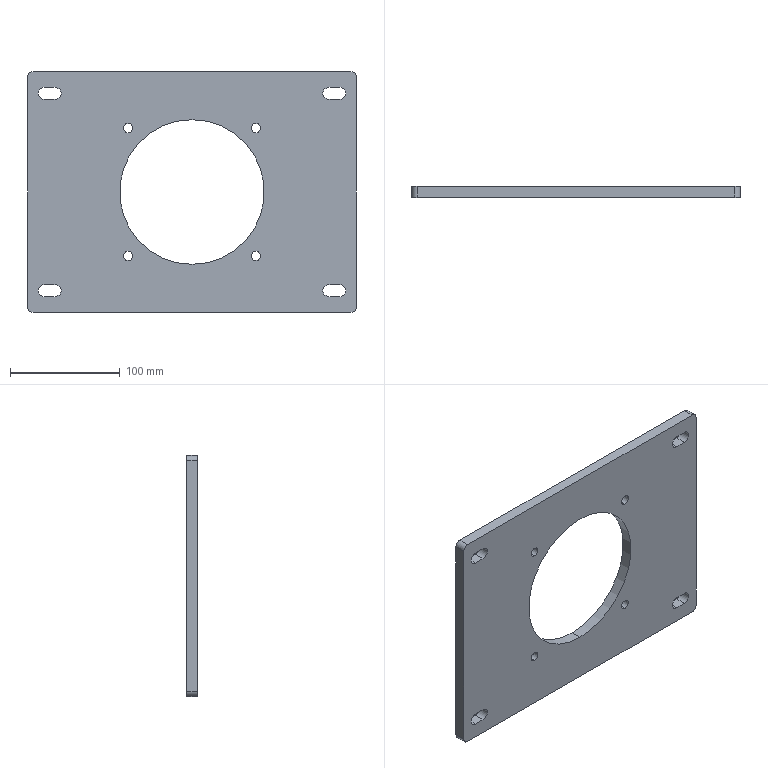Part | SolidWorks | features ICE 2, Extrusion 1, Fillet 1, HoleWzd 1 | 1 solid | 36 faces | box 300 x 10 x 220 mm | volume 512466 mm3 | cylinder 22 | plane 14 | commonest cylinder face diameters 8.5 x8 11 x8 10 x4 132 x2
STEP:
#1=CARTESIAN_POINT('',(-58.336,0.,-62.586));
#2=VERTEX_POINT('',#1);
#3=CARTESIAN_POINT('',(-58.336,0.,-54.086));
#4=VERTEX_POINT('',#3);
#5=CARTESIAN_POINT('',(-58.336,0.,-58.336));
#6=DIRECTION('',(0.,1.,0.));
#7=DIRECTION('',(0.,0.,1.));
#8=AXIS2_PLACEMENT_3D('',#5,#6,#7);
#9=CIRCLE('',#8,4.25);
#10=EDGE_CURVE('',#2,#4,#9,.T.);
#11=ORIENTED_EDGE('',*,*,#10,.F.);
#12=CARTESIAN_POINT('',(-58.336,10.,-62.586));
#13=VERTEX_POINT('',#12);
#14=CARTESIAN_POINT('',(-58.336,10.,-62.586));
#15=DIRECTION('',(0.,1.,0.));
#16=VECTOR('',#15,1000.);
#17=LINE('',#14,#16);
#18=EDGE_CURVE('',#2,#13,#17,.T.);
#19=ORIENTED_EDGE('',*,*,#18,.T.);
#20=CARTESIAN_POINT('',(-58.336,10.,-54.086));
#21=VERTEX_POINT('',#20);
#22=CARTESIAN_POINT('',(-58.336,10.,-58.336));
#23=DIRECTION('',(0.,1.,0.));
#24=DIRECTION('',(0.,0.,1.));
#25=AXIS2_PLACEMENT_3D('',#22,#23,#24);
#26=CIRCLE('',#25,4.25);
#27=EDGE_CURVE('',#13,#21,#26,.T.);
#28=ORIENTED_EDGE('',*,*,#27,.T.);
#29=CARTESIAN_POINT('',(-58.336,10.,-54.086));
#30=DIRECTION('',(0.,1.,0.));
#31=VECTOR('',#30,1000.);
#32=LINE('',#29,#31);
#33=EDGE_CURVE('',#4,#21,#32,.T.);
#34=ORIENTED_EDGE('',*,*,#33,.F.);
#35=EDGE_LOOP('',(#11,#19,#28,#34));
#36=FACE_OUTER_BOUND('',#35,.T.);
#37=CARTESIAN_POINT('',(-58.336,10.,-58.336));
#38=DIRECTION('',(0.,1.,0.));
#39=DIRECTION('',(0.,0.,1.));
#40=AXIS2_PLACEMENT_3D('',#37,#38,#39);
#41=CYLINDRICAL_SURFACE('',#40,4.25);
#42=ADVANCED_FACE('',(#36),#41,.F.);
#43=CARTESIAN_POINT('',(58.336,0.,-62.586));
#44=VERTEX_POINT('',#43);
#45=CARTESIAN_POINT('',(58.336,0.,-54.086));
#46=VERTEX_POINT('',#45);
#47=CARTESIAN_POINT('',(58.336,0.,-58.336));
#48=DIRECTION('',(0.,1.,0.));
#49=DIRECTION('',(0.,0.,1.));
#50=AXIS2_PLACEMENT_3D('',#47,#48,#49);
#51=CIRCLE('',#50,4.25);
#52=EDGE_CURVE('',#44,#46,#51,.T.);
#53=ORIENTED_EDGE('',*,*,#52,.F.);
#54=CARTESIAN_POINT('',(58.336,10.,-62.586));
#55=VERTEX_POINT('',#54);
#56=CARTESIAN_POINT('',(58.336,10.,-62.586));
#57=DIRECTION('',(0.,1.,0.));
#58=VECTOR('',#57,1000.);
#59=LINE('',#56,#58);
#60=EDGE_CURVE('',#44,#55,#59,.T.);
#61=ORIENTED_EDGE('',*,*,#60,.T.);
#62=CARTESIAN_POINT('',(58.336,10.,-54.086));
#63=VERTEX_POINT('',#62);
#64=CARTESIAN_POINT('',(58.336,10.,-58.336));
#65=DIRECTION('',(0.,1.,0.));
#66=DIRECTION('',(0.,0.,1.));
#67=AXIS2_PLACEMENT_3D('',#64,#65,#66);
#68=CIRCLE('',#67,4.25);
#69=EDGE_CURVE('',#55,#63,#68,.T.);
#70=ORIENTED_EDGE('',*,*,#69,.T.);
#71=CARTESIAN_POINT('',(58.336,10.,-54.086));
#72=DIRECTION('',(0.,1.,0.));
#73=VECTOR('',#72,1000.);
#74=LINE('',#71,#73);
#75=EDGE_CURVE('',#46,#63,#74,.T.);
#76=ORIENTED_EDGE('',*,*,#75,.F.);
#77=EDGE_LOOP('',(#53,#61,#70,#76));
#78=FACE_OUTER_BOUND('',#77,.T.);
#79=CARTESIAN_POINT('',(58.336,10.,-58.336));
#80=DIRECTION('',(0.,1.,0.));
#81=DIRECTION('',(0.,0.,1.));
#82=AXIS2_PLACEMENT_3D('',#79,#80,#81);
#83=CYLINDRICAL_SURFACE('',#82,4.25);
#84=ADVANCED_FACE('',(#78),#83,.F.);
#85=CARTESIAN_POINT('',(58.336,0.,54.086));
#86=VERTEX_POINT('',#85);
#87=CARTESIAN_POINT('',(58.336,0.,62.586));
#88=VERTEX_POINT('',#87);
#89=CARTESIAN_POINT('',(58.336,0.,58.336));
#90=DIRECTION('',(0.,1.,0.));
#91=DIRECTION('',(0.,0.,1.));
#92=AXIS2_PLACEMENT_3D('',#89,#90,#91);
#93=CIRCLE('',#92,4.25);
#94=EDGE_CURVE('',#86,#88,#93,.T.);
#95=ORIENTED_EDGE('',*,*,#94,.F.);
#96=CARTESIAN_POINT('',(58.336,10.,54.086));
#97=VERTEX_POINT('',#96);
#98=CARTESIAN_POINT('',(58.336,10.,54.086));
#99=DIRECTION('',(0.,1.,0.));
#100=VECTOR('',#99,1000.);
#101=LINE('',#98,#100);
#102=EDGE_CURVE('',#86,#97,#101,.T.);
#103=ORIENTED_EDGE('',*,*,#102,.T.);
#104=CARTESIAN_POINT('',(58.336,10.,62.586));
#105=VERTEX_POINT('',#104);
#106=CARTESIAN_POINT('',(58.336,10.,58.336));
#107=DIRECTION('',(0.,1.,0.));
#108=DIRECTION('',(0.,0.,1.));
#109=AXIS2_PLACEMENT_3D('',#106,#107,#108);
#110=CIRCLE('',#109,4.25);
#111=EDGE_CURVE('',#97,#105,#110,.T.);
#112=ORIENTED_EDGE('',*,*,#111,.T.);
#113=CARTESIAN_POINT('',(58.336,10.,62.586));
#114=DIRECTION('',(0.,1.,0.));
#115=VECTOR('',#114,1000.);
#116=LINE('',#113,#115);
#117=EDGE_CURVE('',#88,#105,#116,.T.);
#118=ORIENTED_EDGE('',*,*,#117,.F.);
#119=EDGE_LOOP('',(#95,#103,#112,#118));
#120=FACE_OUTER_BOUND('',#119,.T.);
#121=CARTESIAN_POINT('',(58.336,10.,58.336));
#122=DIRECTION('',(0.,1.,0.));
#123=DIRECTION('',(0.,0.,1.));
#124=AXIS2_PLACEMENT_3D('',#121,#122,#123);
#125=CYLINDRICAL_SURFACE('',#124,4.25);
#126=ADVANCED_FACE('',(#120),#125,.F.);
#127=CARTESIAN_POINT('',(-58.336,0.,54.086));
#128=VERTEX_POINT('',#127);
#129=CARTESIAN_POINT('',(-58.336,0.,62.586));
#130=VERTEX_POINT('',#129);
#131=CARTESIAN_POINT('',(-58.336,0.,58.336));
#132=DIRECTION('',(0.,1.,0.));
#133=DIRECTION('',(0.,0.,1.));
#134=AXIS2_PLACEMENT_3D('',#131,#132,#133);
#135=CIRCLE('',#134,4.25);
#136=EDGE_CURVE('',#128,#130,#135,.T.);
#137=ORIENTED_EDGE('',*,*,#136,.F.);
#138=CARTESIAN_POINT('',(-58.336,10.,54.086));
#139=VERTEX_POINT('',#138);
#140=CARTESIAN_POINT('',(-58.336,10.,54.086));
#141=DIRECTION('',(0.,1.,0.));
#142=VECTOR('',#141,1000.);
#143=LINE('',#140,#142);
#144=EDGE_CURVE('',#128,#139,#143,.T.);
#145=ORIENTED_EDGE('',*,*,#144,.T.);
#146=CARTESIAN_POINT('',(-58.336,10.,62.586));
#147=VERTEX_POINT('',#146);
#148=CARTESIAN_POINT('',(-58.336,10.,58.336));
#149=DIRECTION('',(0.,1.,0.));
#150=DIRECTION('',(0.,0.,1.));
#151=AXIS2_PLACEMENT_3D('',#148,#149,#150);
#152=CIRCLE('',#151,4.25);
#153=EDGE_CURVE('',#139,#147,#152,.T.);
#154=ORIENTED_EDGE('',*,*,#153,.T.);
#155=CARTESIAN_POINT('',(-58.336,10.,62.586));
#156=DIRECTION('',(0.,1.,0.));
#157=VECTOR('',#156,1000.);
#158=LINE('',#155,#157);
#159=EDGE_CURVE('',#130,#147,#158,.T.);
#160=ORIENTED_EDGE('',*,*,#159,.F.);
#161=EDGE_LOOP('',(#137,#145,#154,#160));
#162=FACE_OUTER_BOUND('',#161,.T.);
#163=CARTESIAN_POINT('',(-58.336,10.,58.336));
#164=DIRECTION('',(0.,1.,0.));
#165=DIRECTION('',(0.,0.,1.));
#166=AXIS2_PLACEMENT_3D('',#163,#164,#165);
#167=CYLINDRICAL_SURFACE('',#166,4.25);
#168=ADVANCED_FACE('',(#162),#167,.F.);
#169=CARTESIAN_POINT('',(0.,0.,-66.));
#170=VERTEX_POINT('',#169);
#171=CARTESIAN_POINT('',(0.,0.,66.));
#172=VERTEX_POINT('',#171);
#173=CARTESIAN_POINT('',(0.,0.,0.));
#174=DIRECTION('',(0.,1.,0.));
#175=DIRECTION('',(0.,0.,1.));
#176=AXIS2_PLACEMENT_3D('',#173,#174,#175);
#177=CIRCLE('',#176,66.);
#178=EDGE_CURVE('',#170,#172,#177,.T.);
#179=ORIENTED_EDGE('',*,*,#178,.F.);
#180=CARTESIAN_POINT('',(0.,10.,-66.));
#181=VERTEX_POINT('',#180);
#182=CARTESIAN_POINT('',(0.,0.,-66.));
#183=DIRECTION('',(0.,1.,0.));
#184=VECTOR('',#183,1000.);
#185=LINE('',#182,#184);
#186=EDGE_CURVE('',#170,#181,#185,.T.);
#187=ORIENTED_EDGE('',*,*,#186,.T.);
#188=CARTESIAN_POINT('',(0.,10.,66.));
#189=VERTEX_POINT('',#188);
#190=CARTESIAN_POINT('',(0.,10.,0.));
#191=DIRECTION('',(0.,1.,0.));
#192=DIRECTION('',(0.,0.,1.));
#193=AXIS2_PLACEMENT_3D('',#190,#191,#192);
#194=CIRCLE('',#193,66.);
#195=EDGE_CURVE('',#181,#189,#194,.T.);
#196=ORIENTED_EDGE('',*,*,#195,.T.);
#197=CARTESIAN_POINT('',(0.,0.,66.));
#198=DIRECTION('',(0.,1.,0.));
#199=VECTOR('',#198,1000.);
#200=LINE('',#197,#199);
#201=EDGE_CURVE('',#172,#189,#200,.T.);
#202=ORIENTED_EDGE('',*,*,#201,.F.);
#203=EDGE_LOOP('',(#179,#187,#196,#202));
#204=FACE_OUTER_BOUND('',#203,.T.);
#205=CARTESIAN_POINT('',(0.,0.,0.));
#206=DIRECTION('',(0.,1.,0.));
#207=DIRECTION('',(0.,0.,1.));
#208=AXIS2_PLACEMENT_3D('',#205,#206,#207);
#209=CYLINDRICAL_SURFACE('',#208,66.);
#210=ADVANCED_FACE('',(#204),#209,.F.);
#211=CARTESIAN_POINT('',(150.,10.,105.));
#212=VERTEX_POINT('',#211);
#213=CARTESIAN_POINT('',(150.,10.,-105.));
#214=VERTEX_POINT('',#213);
#215=CARTESIAN_POINT('',(150.,10.,-110.));
#216=DIRECTION('',(0.,0.,-1.));
#217=VECTOR('',#216,1000.);
#218=LINE('',#215,#217);
#219=EDGE_CURVE('',#212,#214,#218,.T.);
#220=ORIENTED_EDGE('',*,*,#219,.F.);
#221=CARTESIAN_POINT('',(150.,0.,105.));
#222=VERTEX_POINT('',#221);
#223=CARTESIAN_POINT('',(150.,10.,105.));
#224=DIRECTION('',(0.,-1.,0.));
#225=VECTOR('',#224,1000.);
#226=LINE('',#223,#225);
#227=EDGE_CURVE('',#212,#222,#226,.T.);
#228=ORIENTED_EDGE('',*,*,#227,.T.);
#229=CARTESIAN_POINT('',(150.,0.,-105.));
#230=VERTEX_POINT('',#229);
#231=CARTESIAN_POINT('',(150.,0.,-110.));
#232=DIRECTION('',(0.,0.,-1.));
#233=VECTOR('',#232,1000.);
#234=LINE('',#231,#233);
#235=EDGE_CURVE('',#222,#230,#234,.T.);
#236=ORIENTED_EDGE('',*,*,#235,.T.);
#237=CARTESIAN_POINT('',(150.,10.,-105.));
#238=DIRECTION('',(0.,1.,0.));
#239=VECTOR('',#238,1000.);
#240=LINE('',#237,#239);
#241=EDGE_CURVE('',#230,#214,#240,.T.);
#242=ORIENTED_EDGE('',*,*,#241,.T.);
#243=EDGE_LOOP('',(#220,#228,#236,#242));
#244=FACE_OUTER_BOUND('',#243,.T.);
#245=CARTESIAN_POINT('',(150.,10.,-110.));
#246=DIRECTION('',(-1.,0.,0.));
#247=DIRECTION('',(0.,0.,1.));
#248=AXIS2_PLACEMENT_3D('',#245,#246,#247);
#249=PLANE('',#248);
#250=ADVANCED_FACE('',(#244),#249,.F.);
#251=CARTESIAN_POINT('',(145.,10.,-110.));
#252=VERTEX_POINT('',#251);
#253=CARTESIAN_POINT('',(-145.,10.,-110.));
#254=VERTEX_POINT('',#253);
#255=CARTESIAN_POINT('',(-150.,10.,-110.));
#256=DIRECTION('',(-1.,0.,0.));
#257=VECTOR('',#256,1000.);
#258=LINE('',#255,#257);
#259=EDGE_CURVE('',#252,#254,#258,.T.);
#260=ORIENTED_EDGE('',*,*,#259,.F.);
#261=CARTESIAN_POINT('',(145.,0.,-110.));
#262=VERTEX_POINT('',#261);
#263=CARTESIAN_POINT('',(145.,10.,-110.));
#264=DIRECTION('',(0.,-1.,0.));
#265=VECTOR('',#264,1000.);
#266=LINE('',#263,#265);
#267=EDGE_CURVE('',#252,#262,#266,.T.);
#268=ORIENTED_EDGE('',*,*,#267,.T.);
#269=CARTESIAN_POINT('',(-145.,0.,-110.));
#270=VERTEX_POINT('',#269);
#271=CARTESIAN_POINT('',(-150.,0.,-110.));
#272=DIRECTION('',(-1.,0.,0.));
#273=VECTOR('',#272,1000.);
#274=LINE('',#271,#273);
#275=EDGE_CURVE('',#262,#270,#274,.T.);
#276=ORIENTED_EDGE('',*,*,#275,.T.);
#277=CARTESIAN_POINT('',(-145.,10.,-110.));
#278=DIRECTION('',(0.,1.,0.));
#279=VECTOR('',#278,1000.);
#280=LINE('',#277,#279);
#281=EDGE_CURVE('',#270,#254,#280,.T.);
#282=ORIENTED_EDGE('',*,*,#281,.T.);
#283=EDGE_LOOP('',(#260,#268,#276,#282));
#284=FACE_OUTER_BOUND('',#283,.T.);
#285=CARTESIAN_POINT('',(-150.,10.,-110.));
#286=DIRECTION('',(0.,0.,1.));
#287=DIRECTION('',(1.,0.,0.));
#288=AXIS2_PLACEMENT_3D('',#285,#286,#287);
#289=PLANE('',#288);
#290=ADVANCED_FACE('',(#284),#289,.F.);
#291=CARTESIAN_POINT('',(-150.,10.,-105.));
#292=VERTEX_POINT('',#291);
#293=CARTESIAN_POINT('',(-150.,10.,105.));
#294=VERTEX_POINT('',#293);
#295=CARTESIAN_POINT('',(-150.,10.,-110.));
#296=DIRECTION('',(0.,0.,1.));
#297=VECTOR('',#296,1000.);
#298=LINE('',#295,#297);
#299=EDGE_CURVE('',#292,#294,#298,.T.);
#300=ORIENTED_EDGE('',*,*,#299,.F.);
#301=CARTESIAN_POINT('',(-150.,0.,-105.));
#302=VERTEX_POINT('',#301);
#303=CARTESIAN_POINT('',(-150.,10.,-105.));
#304=DIRECTION('',(0.,-1.,0.));
#305=VECTOR('',#304,1000.);
#306=LINE('',#303,#305);
#307=EDGE_CURVE('',#292,#302,#306,.T.);
#308=ORIENTED_EDGE('',*,*,#307,.T.);
#309=CARTESIAN_POINT('',(-150.,0.,105.));
#310=VERTEX_POINT('',#309);
#311=CARTESIAN_POINT('',(-150.,0.,-110.));
#312=DIRECTION('',(0.,0.,1.));
#313=VECTOR('',#312,1000.);
#314=LINE('',#311,#313);
#315=EDGE_CURVE('',#302,#310,#314,.T.);
#316=ORIENTED_EDGE('',*,*,#315,.T.);
#317=CARTESIAN_POINT('',(-150.,10.,105.));
#318=DIRECTION('',(0.,1.,0.));
#319=VECTOR('',#318,1000.);
#320=LINE('',#317,#319);
#321=EDGE_CURVE('',#310,#294,#320,.T.);
#322=ORIENTED_EDGE('',*,*,#321,.T.);
#323=EDGE_LOOP('',(#300,#308,#316,#322));
#324=FACE_OUTER_BOUND('',#323,.T.);
#325=CARTESIAN_POINT('',(-150.,10.,-110.));
#326=DIRECTION('',(1.,0.,0.));
#327=DIRECTION('',(0.,0.,-1.));
#328=AXIS2_PLACEMENT_3D('',#325,#326,#327);
#329=PLANE('',#328);
#330=ADVANCED_FACE('',(#324),#329,.F.);
#331=CARTESIAN_POINT('',(-145.,0.,110.));
#332=VERTEX_POINT('',#331);
#333=CARTESIAN_POINT('',(145.,0.,110.));
#334=VERTEX_POINT('',#333);
#335=CARTESIAN_POINT('',(-150.,0.,110.));
#336=DIRECTION('',(1.,0.,0.));
#337=VECTOR('',#336,1000.);
#338=LINE('',#335,#337);
#339=EDGE_CURVE('',#332,#334,#338,.T.);
#340=ORIENTED_EDGE('',*,*,#339,.T.);
#341=CARTESIAN_POINT('',(145.,10.,110.));
#342=VERTEX_POINT('',#341);
#343=CARTESIAN_POINT('',(145.,10.,110.));
#344=DIRECTION('',(0.,1.,0.));
#345=VECTOR('',#344,1000.);
#346=LINE('',#343,#345);
#347=EDGE_CURVE('',#334,#342,#346,.T.);
#348=ORIENTED_EDGE('',*,*,#347,.T.);
#349=CARTESIAN_POINT('',(-145.,10.,110.));
#350=VERTEX_POINT('',#349);
#351=CARTESIAN_POINT('',(-150.,10.,110.));
#352=DIRECTION('',(1.,0.,0.));
#353=VECTOR('',#352,1000.);
#354=LINE('',#351,#353);
#355=EDGE_CURVE('',#350,#342,#354,.T.);
#356=ORIENTED_EDGE('',*,*,#355,.F.);
#357=CARTESIAN_POINT('',(-145.,10.,110.));
#358=DIRECTION('',(0.,-1.,0.));
#359=VECTOR('',#358,1000.);
#360=LINE('',#357,#359);
#361=EDGE_CURVE('',#350,#332,#360,.T.);
#362=ORIENTED_EDGE('',*,*,#361,.T.);
#363=EDGE_LOOP('',(#340,#348,#356,#362));
#364=FACE_OUTER_BOUND('',#363,.T.);
#365=CARTESIAN_POINT('',(-150.,10.,110.));
#366=DIRECTION('',(0.,0.,-1.));
#367=DIRECTION('',(-1.,0.,0.));
#368=AXIS2_PLACEMENT_3D('',#365,#366,#367);
#369=PLANE('',#368);
#370=ADVANCED_FACE('',(#364),#369,.F.);
#371=CARTESIAN_POINT('',(-135.,10.,84.5));
#372=VERTEX_POINT('',#371);
#373=CARTESIAN_POINT('',(-135.,10.,95.5));
#374=VERTEX_POINT('',#373);
#375=CARTESIAN_POINT('',(-135.,10.,90.));
#376=DIRECTION('',(0.,1.,0.));
#377=DIRECTION('',(0.,0.,-1.));
#378=AXIS2_PLACEMENT_3D('',#375,#376,#377);
#379=CIRCLE('',#378,5.5);
#380=EDGE_CURVE('',#372,#374,#379,.T.);
#381=ORIENTED_EDGE('',*,*,#380,.F.);
#382=CARTESIAN_POINT('',(-125.,10.,84.5));
#383=VERTEX_POINT('',#382);
#384=CARTESIAN_POINT('',(-135.,10.,84.5));
#385=DIRECTION('',(-1.,0.,0.));
#386=VECTOR('',#385,1000.);
#387=LINE('',#384,#386);
#388=EDGE_CURVE('',#383,#372,#387,.T.);
#389=ORIENTED_EDGE('',*,*,#388,.F.);
#390=CARTESIAN_POINT('',(-125.,10.,95.5));
#391=VERTEX_POINT('',#390);
#392=CARTESIAN_POINT('',(-125.,10.,90.));
#393=DIRECTION('',(0.,1.,0.));
#394=DIRECTION('',(0.,0.,-1.));
#395=AXIS2_PLACEMENT_3D('',#392,#393,#394);
#396=CIRCLE('',#395,5.5);
#397=EDGE_CURVE('',#391,#383,#396,.T.);
#398=ORIENTED_EDGE('',*,*,#397,.F.);
#399=CARTESIAN_POINT('',(-135.,10.,95.5));
#400=DIRECTION('',(1.,0.,0.));
#401=VECTOR('',#400,1000.);
#402=LINE('',#399,#401);
#403=EDGE_CURVE('',#374,#391,#402,.T.);
#404=ORIENTED_EDGE('',*,*,#403,.F.);
#405=EDGE_LOOP('',(#381,#389,#398,#404));
#406=FACE_BOUND('',#405,.T.);
#407=CARTESIAN_POINT('',(135.,10.,95.5));
#408=VERTEX_POINT('',#407);
#409=CARTESIAN_POINT('',(135.,10.,84.5));
#410=VERTEX_POINT('',#409);
#411=CARTESIAN_POINT('',(135.,10.,90.));
#412=DIRECTION('',(0.,1.,0.));
#413=DIRECTION('',(0.,0.,1.));
#414=AXIS2_PLACEMENT_3D('',#411,#412,#413);
#415=CIRCLE('',#414,5.5);
#416=EDGE_CURVE('',#408,#410,#415,.T.);
#417=ORIENTED_EDGE('',*,*,#416,.F.);
#418=CARTESIAN_POINT('',(125.,10.,95.5));
#419=VERTEX_POINT('',#418);
#420=CARTESIAN_POINT('',(135.,10.,95.5));
#421=DIRECTION('',(1.,0.,0.));
#422=VECTOR('',#421,1000.);
#423=LINE('',#420,#422);
#424=EDGE_CURVE('',#419,#408,#423,.T.);
#425=ORIENTED_EDGE('',*,*,#424,.F.);
#426=CARTESIAN_POINT('',(125.,10.,84.5));
#427=VERTEX_POINT('',#426);
#428=CARTESIAN_POINT('',(125.,10.,90.));
#429=DIRECTION('',(0.,1.,0.));
#430=DIRECTION('',(0.,0.,1.));
#431=AXIS2_PLACEMENT_3D('',#428,#429,#430);
#432=CIRCLE('',#431,5.5);
#433=EDGE_CURVE('',#427,#419,#432,.T.);
#434=ORIENTED_EDGE('',*,*,#433,.F.);
#435=CARTESIAN_POINT('',(135.,10.,84.5));
#436=DIRECTION('',(-1.,0.,0.));
#437=VECTOR('',#436,1000.);
#438=LINE('',#435,#437);
#439=EDGE_CURVE('',#410,#427,#438,.T.);
#440=ORIENTED_EDGE('',*,*,#439,.F.);
#441=EDGE_LOOP('',(#417,#425,#434,#440));
#442=FACE_BOUND('',#441,.T.);
#443=CARTESIAN_POINT('',(135.,10.,-84.5));
#444=VERTEX_POINT('',#443);
#445=CARTESIAN_POINT('',(135.,10.,-95.5));
#446=VERTEX_POINT('',#445);
#447=CARTESIAN_POINT('',(135.,10.,-90.));
#448=DIRECTION('',(0.,1.,0.));
#449=DIRECTION('',(0.,0.,-1.));
#450=AXIS2_PLACEMENT_3D('',#447,#448,#449);
#451=CIRCLE('',#450,5.5);
#452=EDGE_CURVE('',#444,#446,#451,.T.);
#453=ORIENTED_EDGE('',*,*,#452,.F.);
#454=CARTESIAN_POINT('',(125.,10.,-84.5));
#455=VERTEX_POINT('',#454);
#456=CARTESIAN_POINT('',(135.,10.,-84.5));
#457=DIRECTION('',(1.,0.,0.));
#458=VECTOR('',#457,1000.);
#459=LINE('',#456,#458);
#460=EDGE_CURVE('',#455,#444,#459,.T.);
#461=ORIENTED_EDGE('',*,*,#460,.F.);
#462=CARTESIAN_POINT('',(125.,10.,-95.5));
#463=VERTEX_POINT('',#462);
#464=CARTESIAN_POINT('',(125.,10.,-90.));
#465=DIRECTION('',(0.,1.,0.));
#466=DIRECTION('',(0.,0.,-1.));
#467=AXIS2_PLACEMENT_3D('',#464,#465,#466);
#468=CIRCLE('',#467,5.5);
#469=EDGE_CURVE('',#463,#455,#468,.T.);
#470=ORIENTED_EDGE('',*,*,#469,.F.);
#471=CARTESIAN_POINT('',(135.,10.,-95.5));
#472=DIRECTION('',(-1.,0.,0.));
#473=VECTOR('',#472,1000.);
#474=LINE('',#471,#473);
#475=EDGE_CURVE('',#446,#463,#474,.T.);
#476=ORIENTED_EDGE('',*,*,#475,.F.);
#477=EDGE_LOOP('',(#453,#461,#470,#476));
#478=FACE_BOUND('',#477,.T.);
#479=CARTESIAN_POINT('',(-135.,10.,-95.5));
#480=VERTEX_POINT('',#479);
#481=CARTESIAN_POINT('',(-135.,10.,-84.5));
#482=VERTEX_POINT('',#481);
#483=CARTESIAN_POINT('',(-135.,10.,-90.));
#484=DIRECTION('',(0.,1.,0.));
#485=DIRECTION('',(0.,0.,1.));
#486=AXIS2_PLACEMENT_3D('',#483,#484,#485);
#487=CIRCLE('',#486,5.5);
#488=EDGE_CURVE('',#480,#482,#487,.T.);
#489=ORIENTED_EDGE('',*,*,#488,.F.);
#490=CARTESIAN_POINT('',(-125.,10.,-95.5));
#491=VERTEX_POINT('',#490);
#492=CARTESIAN_POINT('',(-135.,10.,-95.5));
#493=DIRECTION('',(-1.,0.,0.));
#494=VECTOR('',#493,1000.);
#495=LINE('',#492,#494);
#496=EDGE_CURVE('',#491,#480,#495,.T.);
#497=ORIENTED_EDGE('',*,*,#496,.F.);
#498=CARTESIAN_POINT('',(-125.,10.,-84.5));
#499=VERTEX_POINT('',#498);
#500=CARTESIAN_POINT('',(-125.,10.,-90.));
#501=DIRECTION('',(0.,1.,0.));
#502=DIRECTION('',(0.,0.,1.));
#503=AXIS2_PLACEMENT_3D('',#500,#501,#502);
#504=CIRCLE('',#503,5.5);
#505=EDGE_CURVE('',#499,#491,#504,.T.);
#506=ORIENTED_EDGE('',*,*,#505,.F.);
#507=CARTESIAN_POINT('',(-135.,10.,-84.5));
#508=DIRECTION('',(1.,0.,0.));
#509=VECTOR('',#508,1000.);
#510=LINE('',#507,#509);
#511=EDGE_CURVE('',#482,#499,#510,.T.);
#512=ORIENTED_EDGE('',*,*,#511,.F.);
#513=EDGE_LOOP('',(#489,#497,#506,#512));
#514=FACE_BOUND('',#513,.T.);
#515=CARTESIAN_POINT('',(-58.336,10.,-58.336));
#516=DIRECTION('',(0.,1.,0.));
#517=DIRECTION('',(0.,0.,1.));
#518=AXIS2_PLACEMENT_3D('',#515,#516,#517);
#519=CIRCLE('',#518,4.25);
#520=EDGE_CURVE('',#21,#13,#519,.T.);
#521=ORIENTED_EDGE('',*,*,#520,.F.);
#522=ORIENTED_EDGE('',*,*,#27,.F.);
#523=EDGE_LOOP('',(#521,#522));
#524=FACE_BOUND('',#523,.T.);
#525=CARTESIAN_POINT('',(58.336,10.,-58.336));
#526=DIRECTION('',(0.,1.,0.));
#527=DIRECTION('',(0.,0.,1.));
#528=AXIS2_PLACEMENT_3D('',#525,#526,#527);
#529=CIRCLE('',#528,4.25);
#530=EDGE_CURVE('',#63,#55,#529,.T.);
#531=ORIENTED_EDGE('',*,*,#530,.F.);
#532=ORIENTED_EDGE('',*,*,#69,.F.);
#533=EDGE_LOOP('',(#531,#532));
#534=FACE_BOUND('',#533,.T.);
#535=CARTESIAN_POINT('',(58.336,10.,58.336));
#536=DIRECTION('',(0.,1.,0.));
#537=DIRECTION('',(0.,0.,1.));
#538=AXIS2_PLACEMENT_3D('',#535,#536,#537);
#539=CIRCLE('',#538,4.25);
#540=EDGE_CURVE('',#105,#97,#539,.T.);
#541=ORIENTED_EDGE('',*,*,#540,.F.);
#542=ORIENTED_EDGE('',*,*,#111,.F.);
#543=EDGE_LOOP('',(#541,#542));
#544=FACE_BOUND('',#543,.T.);
#545=CARTESIAN_POINT('',(-58.336,10.,58.336));
#546=DIRECTION('',(0.,1.,0.));
#547=DIRECTION('',(0.,0.,1.));
#548=AXIS2_PLACEMENT_3D('',#545,#546,#547);
#549=CIRCLE('',#548,4.25);
#550=EDGE_CURVE('',#147,#139,#549,.T.);
#551=ORIENTED_EDGE('',*,*,#550,.F.);
#552=ORIENTED_EDGE('',*,*,#153,.F.);
#553=EDGE_LOOP('',(#551,#552));
#554=FACE_BOUND('',#553,.T.);
#555=CARTESIAN_POINT('',(0.,10.,0.));
#556=DIRECTION('',(0.,1.,0.));
#557=DIRECTION('',(0.,0.,1.));
#558=AXIS2_PLACEMENT_3D('',#555,#556,#557);
#559=CIRCLE('',#558,66.);
#560=EDGE_CURVE('',#189,#181,#559,.T.);
#561=ORIENTED_EDGE('',*,*,#560,.F.);
#562=ORIENTED_EDGE('',*,*,#195,.F.);
#563=EDGE_LOOP('',(#561,#562));
#564=FACE_BOUND('',#563,.T.);
#565=ORIENTED_EDGE('',*,*,#355,.T.);
#566=CARTESIAN_POINT('',(145.,10.,105.));
#567=DIRECTION('',(0.,1.,0.));
#568=DIRECTION('',(0.,0.,1.));
#569=AXIS2_PLACEMENT_3D('',#566,#567,#568);
#570=CIRCLE('',#569,5.);
#571=EDGE_CURVE('',#342,#212,#570,.T.);
#572=ORIENTED_EDGE('',*,*,#571,.T.);
#573=ORIENTED_EDGE('',*,*,#219,.T.);
#574=CARTESIAN_POINT('',(145.,10.,-105.));
#575=DIRECTION('',(0.,1.,0.));
#576=DIRECTION('',(0.,0.,1.));
#577=AXIS2_PLACEMENT_3D('',#574,#575,#576);
#578=CIRCLE('',#577,5.);
#579=EDGE_CURVE('',#214,#252,#578,.T.);
#580=ORIENTED_EDGE('',*,*,#579,.T.);
#581=ORIENTED_EDGE('',*,*,#259,.T.);
#582=CARTESIAN_POINT('',(-145.,10.,-105.));
#583=DIRECTION('',(0.,1.,0.));
#584=DIRECTION('',(0.,0.,1.));
#585=AXIS2_PLACEMENT_3D('',#582,#583,#584);
#586=CIRCLE('',#585,5.);
#587=EDGE_CURVE('',#254,#292,#586,.T.);
#588=ORIENTED_EDGE('',*,*,#587,.T.);
#589=ORIENTED_EDGE('',*,*,#299,.T.);
#590=CARTESIAN_POINT('',(-145.,10.,105.));
#591=DIRECTION('',(0.,1.,0.));
#592=DIRECTION('',(0.,0.,1.));
#593=AXIS2_PLACEMENT_3D('',#590,#591,#592);
#594=CIRCLE('',#593,5.);
#595=EDGE_CURVE('',#294,#350,#594,.T.);
#596=ORIENTED_EDGE('',*,*,#595,.T.);
#597=EDGE_LOOP('',(#565,#572,#573,#580,#581,#588,#589,#596));
#598=FACE_OUTER_BOUND('',#597,.T.);
#599=CARTESIAN_POINT('',(0.,10.,0.));
#600=DIRECTION('',(0.,1.,0.));
#601=DIRECTION('',(0.,0.,1.));
#602=AXIS2_PLACEMENT_3D('',#599,#600,#601);
#603=PLANE('',#602);
#604=ADVANCED_FACE('',(#406,#442,#478,#514,#524,#534,#544,#554,#564,#598),#603,.T.);
#605=CARTESIAN_POINT('',(-125.,0.,84.5));
#606=VERTEX_POINT('',#605);
#607=CARTESIAN_POINT('',(-135.,0.,84.5));
#608=VERTEX_POINT('',#607);
#609=CARTESIAN_POINT('',(-135.,0.,84.5));
#610=DIRECTION('',(-1.,0.,0.));
#611=VECTOR('',#610,1000.);
#612=LINE('',#609,#611);
#613=EDGE_CURVE('',#606,#608,#612,.T.);
#614=ORIENTED_EDGE('',*,*,#613,.T.);
#615=CARTESIAN_POINT('',(-135.,0.,95.5));
#616=VERTEX_POINT('',#615);
#617=CARTESIAN_POINT('',(-135.,0.,90.));
#618=DIRECTION('',(0.,1.,0.));
#619=DIRECTION('',(0.,0.,-1.));
#620=AXIS2_PLACEMENT_3D('',#617,#618,#619);
#621=CIRCLE('',#620,5.5);
#622=EDGE_CURVE('',#608,#616,#621,.T.);
#623=ORIENTED_EDGE('',*,*,#622,.T.);
#624=CARTESIAN_POINT('',(-125.,0.,95.5));
#625=VERTEX_POINT('',#624);
#626=CARTESIAN_POINT('',(-135.,0.,95.5));
#627=DIRECTION('',(1.,0.,0.));
#628=VECTOR('',#627,1000.);
#629=LINE('',#626,#628);
#630=EDGE_CURVE('',#616,#625,#629,.T.);
#631=ORIENTED_EDGE('',*,*,#630,.T.);
#632=CARTESIAN_POINT('',(-125.,0.,90.));
#633=DIRECTION('',(0.,1.,0.));
#634=DIRECTION('',(0.,0.,-1.));
#635=AXIS2_PLACEMENT_3D('',#632,#633,#634);
#636=CIRCLE('',#635,5.5);
#637=EDGE_CURVE('',#625,#606,#636,.T.);
#638=ORIENTED_EDGE('',*,*,#637,.T.);
#639=EDGE_LOOP('',(#614,#623,#631,#638));
#640=FACE_BOUND('',#639,.T.);
#641=CARTESIAN_POINT('',(125.,0.,95.5));
#642=VERTEX_POINT('',#641);
#643=CARTESIAN_POINT('',(135.,0.,95.5));
#644=VERTEX_POINT('',#643);
#645=CARTESIAN_POINT('',(135.,0.,95.5));
#646=DIRECTION('',(1.,0.,0.));
#647=VECTOR('',#646,1000.);
#648=LINE('',#645,#647);
#649=EDGE_CURVE('',#642,#644,#648,.T.);
#650=ORIENTED_EDGE('',*,*,#649,.T.);
#651=CARTESIAN_POINT('',(135.,0.,84.5));
#652=VERTEX_POINT('',#651);
#653=CARTESIAN_POINT('',(135.,0.,90.));
#654=DIRECTION('',(0.,1.,0.));
#655=DIRECTION('',(0.,0.,1.));
#656=AXIS2_PLACEMENT_3D('',#653,#654,#655);
#657=CIRCLE('',#656,5.5);
#658=EDGE_CURVE('',#644,#652,#657,.T.);
#659=ORIENTED_EDGE('',*,*,#658,.T.);
#660=CARTESIAN_POINT('',(125.,0.,84.5));
#661=VERTEX_POINT('',#660);
#662=CARTESIAN_POINT('',(135.,0.,84.5));
#663=DIRECTION('',(-1.,0.,0.));
#664=VECTOR('',#663,1000.);
#665=LINE('',#662,#664);
#666=EDGE_CURVE('',#652,#661,#665,.T.);
#667=ORIENTED_EDGE('',*,*,#666,.T.);
#668=CARTESIAN_POINT('',(125.,0.,90.));
#669=DIRECTION('',(0.,1.,0.));
#670=DIRECTION('',(0.,0.,1.));
#671=AXIS2_PLACEMENT_3D('',#668,#669,#670);
#672=CIRCLE('',#671,5.5);
#673=EDGE_CURVE('',#661,#642,#672,.T.);
#674=ORIENTED_EDGE('',*,*,#673,.T.);
#675=EDGE_LOOP('',(#650,#659,#667,#674));
#676=FACE_BOUND('',#675,.T.);
#677=CARTESIAN_POINT('',(125.,0.,-84.5));
#678=VERTEX_POINT('',#677);
#679=CARTESIAN_POINT('',(135.,0.,-84.5));
#680=VERTEX_POINT('',#679);
#681=CARTESIAN_POINT('',(135.,0.,-84.5));
#682=DIRECTION('',(1.,0.,0.));
#683=VECTOR('',#682,1000.);
#684=LINE('',#681,#683);
#685=EDGE_CURVE('',#678,#680,#684,.T.);
#686=ORIENTED_EDGE('',*,*,#685,.T.);
#687=CARTESIAN_POINT('',(135.,0.,-95.5));
#688=VERTEX_POINT('',#687);
#689=CARTESIAN_POINT('',(135.,0.,-90.));
#690=DIRECTION('',(0.,1.,0.));
#691=DIRECTION('',(0.,0.,-1.));
#692=AXIS2_PLACEMENT_3D('',#689,#690,#691);
#693=CIRCLE('',#692,5.5);
#694=EDGE_CURVE('',#680,#688,#693,.T.);
#695=ORIENTED_EDGE('',*,*,#694,.T.);
#696=CARTESIAN_POINT('',(125.,0.,-95.5));
#697=VERTEX_POINT('',#696);
#698=CARTESIAN_POINT('',(135.,0.,-95.5));
#699=DIRECTION('',(-1.,0.,0.));
#700=VECTOR('',#699,1000.);
#701=LINE('',#698,#700);
#702=EDGE_CURVE('',#688,#697,#701,.T.);
#703=ORIENTED_EDGE('',*,*,#702,.T.);
#704=CARTESIAN_POINT('',(125.,0.,-90.));
#705=DIRECTION('',(0.,1.,0.));
#706=DIRECTION('',(0.,0.,-1.));
#707=AXIS2_PLACEMENT_3D('',#704,#705,#706);
#708=CIRCLE('',#707,5.5);
#709=EDGE_CURVE('',#697,#678,#708,.T.);
#710=ORIENTED_EDGE('',*,*,#709,.T.);
#711=EDGE_LOOP('',(#686,#695,#703,#710));
#712=FACE_BOUND('',#711,.T.);
#713=CARTESIAN_POINT('',(-125.,0.,-95.5));
#714=VERTEX_POINT('',#713);
#715=CARTESIAN_POINT('',(-135.,0.,-95.5));
#716=VERTEX_POINT('',#715);
#717=CARTESIAN_POINT('',(-135.,0.,-95.5));
#718=DIRECTION('',(-1.,0.,0.));
#719=VECTOR('',#718,1000.);
#720=LINE('',#717,#719);
#721=EDGE_CURVE('',#714,#716,#720,.T.);
#722=ORIENTED_EDGE('',*,*,#721,.T.);
#723=CARTESIAN_POINT('',(-135.,0.,-84.5));
#724=VERTEX_POINT('',#723);
#725=CARTESIAN_POINT('',(-135.,0.,-90.));
#726=DIRECTION('',(0.,1.,0.));
#727=DIRECTION('',(0.,0.,1.));
#728=AXIS2_PLACEMENT_3D('',#725,#726,#727);
#729=CIRCLE('',#728,5.5);
#730=EDGE_CURVE('',#716,#724,#729,.T.);
#731=ORIENTED_EDGE('',*,*,#730,.T.);
#732=CARTESIAN_POINT('',(-125.,0.,-84.5));
#733=VERTEX_POINT('',#732);
#734=CARTESIAN_POINT('',(-135.,0.,-84.5));
#735=DIRECTION('',(1.,0.,0.));
#736=VECTOR('',#735,1000.);
#737=LINE('',#734,#736);
#738=EDGE_CURVE('',#724,#733,#737,.T.);
#739=ORIENTED_EDGE('',*,*,#738,.T.);
#740=CARTESIAN_POINT('',(-125.,0.,-90.));
#741=DIRECTION('',(0.,1.,0.));
#742=DIRECTION('',(0.,0.,1.));
#743=AXIS2_PLACEMENT_3D('',#740,#741,#742);
#744=CIRCLE('',#743,5.5);
#745=EDGE_CURVE('',#733,#714,#744,.T.);
#746=ORIENTED_EDGE('',*,*,#745,.T.);
#747=EDGE_LOOP('',(#722,#731,#739,#746));
#748=FACE_BOUND('',#747,.T.);
#749=CARTESIAN_POINT('',(-58.336,0.,-58.336));
#750=DIRECTION('',(0.,1.,0.));
#751=DIRECTION('',(0.,0.,1.));
#752=AXIS2_PLACEMENT_3D('',#749,#750,#751);
#753=CIRCLE('',#752,4.25);
#754=EDGE_CURVE('',#4,#2,#753,.T.);
#755=ORIENTED_EDGE('',*,*,#754,.T.);
#756=ORIENTED_EDGE('',*,*,#10,.T.);
#757=EDGE_LOOP('',(#755,#756));
#758=FACE_BOUND('',#757,.T.);
#759=CARTESIAN_POINT('',(58.336,0.,-58.336));
#760=DIRECTION('',(0.,1.,0.));
#761=DIRECTION('',(0.,0.,1.));
#762=AXIS2_PLACEMENT_3D('',#759,#760,#761);
#763=CIRCLE('',#762,4.25);
#764=EDGE_CURVE('',#46,#44,#763,.T.);
#765=ORIENTED_EDGE('',*,*,#764,.T.);
#766=ORIENTED_EDGE('',*,*,#52,.T.);
#767=EDGE_LOOP('',(#765,#766));
#768=FACE_BOUND('',#767,.T.);
#769=CARTESIAN_POINT('',(58.336,0.,58.336));
#770=DIRECTION('',(0.,1.,0.));
#771=DIRECTION('',(0.,0.,1.));
#772=AXIS2_PLACEMENT_3D('',#769,#770,#771);
#773=CIRCLE('',#772,4.25);
#774=EDGE_CURVE('',#88,#86,#773,.T.);
#775=ORIENTED_EDGE('',*,*,#774,.T.);
#776=ORIENTED_EDGE('',*,*,#94,.T.);
#777=EDGE_LOOP('',(#775,#776));
#778=FACE_BOUND('',#777,.T.);
#779=CARTESIAN_POINT('',(-58.336,0.,58.336));
#780=DIRECTION('',(0.,1.,0.));
#781=DIRECTION('',(0.,0.,1.));
#782=AXIS2_PLACEMENT_3D('',#779,#780,#781);
#783=CIRCLE('',#782,4.25);
#784=EDGE_CURVE('',#130,#128,#783,.T.);
#785=ORIENTED_EDGE('',*,*,#784,.T.);
#786=ORIENTED_EDGE('',*,*,#136,.T.);
#787=EDGE_LOOP('',(#785,#786));
#788=FACE_BOUND('',#787,.T.);
#789=CARTESIAN_POINT('',(0.,0.,0.));
#790=DIRECTION('',(0.,1.,0.));
#791=DIRECTION('',(0.,0.,1.));
#792=AXIS2_PLACEMENT_3D('',#789,#790,#791);
#793=CIRCLE('',#792,66.);
#794=EDGE_CURVE('',#172,#170,#793,.T.);
#795=ORIENTED_EDGE('',*,*,#794,.T.);
#796=ORIENTED_EDGE('',*,*,#178,.T.);
#797=EDGE_LOOP('',(#795,#796));
#798=FACE_BOUND('',#797,.T.);
#799=ORIENTED_EDGE('',*,*,#235,.F.);
#800=CARTESIAN_POINT('',(145.,0.,105.));
#801=DIRECTION('',(0.,-1.,0.));
#802=DIRECTION('',(0.,0.,1.));
#803=AXIS2_PLACEMENT_3D('',#800,#801,#802);
#804=CIRCLE('',#803,5.);
#805=EDGE_CURVE('',#222,#334,#804,.T.);
#806=ORIENTED_EDGE('',*,*,#805,.T.);
#807=ORIENTED_EDGE('',*,*,#339,.F.);
#808=CARTESIAN_POINT('',(-145.,0.,105.));
#809=DIRECTION('',(0.,-1.,0.));
#810=DIRECTION('',(0.,0.,1.));
#811=AXIS2_PLACEMENT_3D('',#808,#809,#810);
#812=CIRCLE('',#811,5.);
#813=EDGE_CURVE('',#332,#310,#812,.T.);
#814=ORIENTED_EDGE('',*,*,#813,.T.);
#815=ORIENTED_EDGE('',*,*,#315,.F.);
#816=CARTESIAN_POINT('',(-145.,0.,-105.));
#817=DIRECTION('',(0.,-1.,0.));
#818=DIRECTION('',(0.,0.,1.));
#819=AXIS2_PLACEMENT_3D('',#816,#817,#818);
#820=CIRCLE('',#819,5.);
#821=EDGE_CURVE('',#302,#270,#820,.T.);
#822=ORIENTED_EDGE('',*,*,#821,.T.);
#823=ORIENTED_EDGE('',*,*,#275,.F.);
#824=CARTESIAN_POINT('',(145.,0.,-105.));
#825=DIRECTION('',(0.,-1.,0.));
#826=DIRECTION('',(0.,0.,1.));
#827=AXIS2_PLACEMENT_3D('',#824,#825,#826);
#828=CIRCLE('',#827,5.);
#829=EDGE_CURVE('',#262,#230,#828,.T.);
#830=ORIENTED_EDGE('',*,*,#829,.T.);
#831=EDGE_LOOP('',(#799,#806,#807,#814,#815,#822,#823,#830));
#832=FACE_OUTER_BOUND('',#831,.T.);
#833=CARTESIAN_POINT('',(0.,0.,0.));
#834=DIRECTION('',(0.,1.,0.));
#835=DIRECTION('',(0.,0.,1.));
#836=AXIS2_PLACEMENT_3D('',#833,#834,#835);
#837=PLANE('',#836);
#838=ADVANCED_FACE('',(#640,#676,#712,#748,#758,#768,#778,#788,#798,#832),#837,.F.);
#839=ORIENTED_EDGE('',*,*,#186,.F.);
#840=ORIENTED_EDGE('',*,*,#794,.F.);
#841=ORIENTED_EDGE('',*,*,#201,.T.);
#842=ORIENTED_EDGE('',*,*,#560,.T.);
#843=EDGE_LOOP('',(#839,#840,#841,#842));
#844=FACE_OUTER_BOUND('',#843,.T.);
#845=CARTESIAN_POINT('',(0.,0.,0.));
#846=DIRECTION('',(0.,1.,0.));
#847=DIRECTION('',(0.,0.,1.));
#848=AXIS2_PLACEMENT_3D('',#845,#846,#847);
#849=CYLINDRICAL_SURFACE('',#848,66.);
#850=ADVANCED_FACE('',(#844),#849,.F.);
#851=ORIENTED_EDGE('',*,*,#144,.F.);
#852=ORIENTED_EDGE('',*,*,#784,.F.);
#853=ORIENTED_EDGE('',*,*,#159,.T.);
#854=ORIENTED_EDGE('',*,*,#550,.T.);
#855=EDGE_LOOP('',(#851,#852,#853,#854));
#856=FACE_OUTER_BOUND('',#855,.T.);
#857=CARTESIAN_POINT('',(-58.336,10.,58.336));
#858=DIRECTION('',(0.,1.,0.));
#859=DIRECTION('',(0.,0.,1.));
#860=AXIS2_PLACEMENT_3D('',#857,#858,#859);
#861=CYLINDRICAL_SURFACE('',#860,4.25);
#862=ADVANCED_FACE('',(#856),#861,.F.);
#863=ORIENTED_EDGE('',*,*,#102,.F.);
#864=ORIENTED_EDGE('',*,*,#774,.F.);
#865=ORIENTED_EDGE('',*,*,#117,.T.);
#866=ORIENTED_EDGE('',*,*,#540,.T.);
#867=EDGE_LOOP('',(#863,#864,#865,#866));
#868=FACE_OUTER_BOUND('',#867,.T.);
#869=CARTESIAN_POINT('',(58.336,10.,58.336));
#870=DIRECTION('',(0.,1.,0.));
#871=DIRECTION('',(0.,0.,1.));
#872=AXIS2_PLACEMENT_3D('',#869,#870,#871);
#873=CYLINDRICAL_SURFACE('',#872,4.25);
#874=ADVANCED_FACE('',(#868),#873,.F.);
#875=ORIENTED_EDGE('',*,*,#60,.F.);
#876=ORIENTED_EDGE('',*,*,#764,.F.);
#877=ORIENTED_EDGE('',*,*,#75,.T.);
#878=ORIENTED_EDGE('',*,*,#530,.T.);
#879=EDGE_LOOP('',(#875,#876,#877,#878));
#880=FACE_OUTER_BOUND('',#879,.T.);
#881=CARTESIAN_POINT('',(58.336,10.,-58.336));
#882=DIRECTION('',(0.,1.,0.));
#883=DIRECTION('',(0.,0.,1.));
#884=AXIS2_PLACEMENT_3D('',#881,#882,#883);
#885=CYLINDRICAL_SURFACE('',#884,4.25);
#886=ADVANCED_FACE('',(#880),#885,.F.);
#887=ORIENTED_EDGE('',*,*,#18,.F.);
#888=ORIENTED_EDGE('',*,*,#754,.F.);
#889=ORIENTED_EDGE('',*,*,#33,.T.);
#890=ORIENTED_EDGE('',*,*,#520,.T.);
#891=EDGE_LOOP('',(#887,#888,#889,#890));
#892=FACE_OUTER_BOUND('',#891,.T.);
#893=CARTESIAN_POINT('',(-58.336,10.,-58.336));
#894=DIRECTION('',(0.,1.,0.));
#895=DIRECTION('',(0.,0.,1.));
#896=AXIS2_PLACEMENT_3D('',#893,#894,#895);
#897=CYLINDRICAL_SURFACE('',#896,4.25);
#898=ADVANCED_FACE('',(#892),#897,.F.);
#899=ORIENTED_EDGE('',*,*,#488,.T.);
#900=CARTESIAN_POINT('',(-135.,0.,-84.5));
#901=DIRECTION('',(0.,1.,0.));
#902=VECTOR('',#901,1000.);
#903=LINE('',#900,#902);
#904=EDGE_CURVE('',#724,#482,#903,.T.);
#905=ORIENTED_EDGE('',*,*,#904,.F.);
#906=ORIENTED_EDGE('',*,*,#730,.F.);
#907=CARTESIAN_POINT('',(-135.,0.,-95.5));
#908=DIRECTION('',(0.,1.,0.));
#909=VECTOR('',#908,1000.);
#910=LINE('',#907,#909);
#911=EDGE_CURVE('',#716,#480,#910,.T.);
#912=ORIENTED_EDGE('',*,*,#911,.T.);
#913=EDGE_LOOP('',(#899,#905,#906,#912));
#914=FACE_OUTER_BOUND('',#913,.T.);
#915=CARTESIAN_POINT('',(-135.,0.,-90.));
#916=DIRECTION('',(0.,1.,0.));
#917=DIRECTION('',(0.,0.,1.));
#918=AXIS2_PLACEMENT_3D('',#915,#916,#917);
#919=CYLINDRICAL_SURFACE('',#918,5.5);
#920=ADVANCED_FACE('',(#914),#919,.F.);
#921=ORIENTED_EDGE('',*,*,#496,.T.);
#922=ORIENTED_EDGE('',*,*,#911,.F.);
#923=ORIENTED_EDGE('',*,*,#721,.F.);
#924=CARTESIAN_POINT('',(-125.,0.,-95.5));
#925=DIRECTION('',(0.,1.,0.));
#926=VECTOR('',#925,1000.);
#927=LINE('',#924,#926);
#928=EDGE_CURVE('',#714,#491,#927,.T.);
#929=ORIENTED_EDGE('',*,*,#928,.T.);
#930=EDGE_LOOP('',(#921,#922,#923,#929));
#931=FACE_OUTER_BOUND('',#930,.T.);
#932=CARTESIAN_POINT('',(-135.,0.,-95.5));
#933=DIRECTION('',(0.,0.,-1.));
#934=DIRECTION('',(-1.,0.,0.));
#935=AXIS2_PLACEMENT_3D('',#932,#933,#934);
#936=PLANE('',#935);
#937=ADVANCED_FACE('',(#931),#936,.F.);
#938=ORIENTED_EDGE('',*,*,#505,.T.);
#939=ORIENTED_EDGE('',*,*,#928,.F.);
#940=ORIENTED_EDGE('',*,*,#745,.F.);
#941=CARTESIAN_POINT('',(-125.,0.,-84.5));
#942=DIRECTION('',(0.,1.,0.));
#943=VECTOR('',#942,1000.);
#944=LINE('',#941,#943);
#945=EDGE_CURVE('',#733,#499,#944,.T.);
#946=ORIENTED_EDGE('',*,*,#945,.T.);
#947=EDGE_LOOP('',(#938,#939,#940,#946));
#948=FACE_OUTER_BOUND('',#947,.T.);
#949=CARTESIAN_POINT('',(-125.,0.,-90.));
#950=DIRECTION('',(0.,1.,0.));
#951=DIRECTION('',(0.,0.,1.));
#952=AXIS2_PLACEMENT_3D('',#949,#950,#951);
#953=CYLINDRICAL_SURFACE('',#952,5.5);
#954=ADVANCED_FACE('',(#948),#953,.F.);
#955=ORIENTED_EDGE('',*,*,#511,.T.);
#956=ORIENTED_EDGE('',*,*,#945,.F.);
#957=ORIENTED_EDGE('',*,*,#738,.F.);
#958=ORIENTED_EDGE('',*,*,#904,.T.);
#959=EDGE_LOOP('',(#955,#956,#957,#958));
#960=FACE_OUTER_BOUND('',#959,.T.);
#961=CARTESIAN_POINT('',(-135.,0.,-84.5));
#962=DIRECTION('',(0.,0.,1.));
#963=DIRECTION('',(1.,0.,0.));
#964=AXIS2_PLACEMENT_3D('',#961,#962,#963);
#965=PLANE('',#964);
#966=ADVANCED_FACE('',(#960),#965,.F.);
#967=ORIENTED_EDGE('',*,*,#452,.T.);
#968=CARTESIAN_POINT('',(135.,0.,-95.5));
#969=DIRECTION('',(0.,1.,0.));
#970=VECTOR('',#969,1000.);
#971=LINE('',#968,#970);
#972=EDGE_CURVE('',#688,#446,#971,.T.);
#973=ORIENTED_EDGE('',*,*,#972,.F.);
#974=ORIENTED_EDGE('',*,*,#694,.F.);
#975=CARTESIAN_POINT('',(135.,0.,-84.5));
#976=DIRECTION('',(0.,1.,0.));
#977=VECTOR('',#976,1000.);
#978=LINE('',#975,#977);
#979=EDGE_CURVE('',#680,#444,#978,.T.);
#980=ORIENTED_EDGE('',*,*,#979,.T.);
#981=EDGE_LOOP('',(#967,#973,#974,#980));
#982=FACE_OUTER_BOUND('',#981,.T.);
#983=CARTESIAN_POINT('',(135.,0.,-90.));
#984=DIRECTION('',(0.,1.,0.));
#985=DIRECTION('',(0.,0.,1.));
#986=AXIS2_PLACEMENT_3D('',#983,#984,#985);
#987=CYLINDRICAL_SURFACE('',#986,5.5);
#988=ADVANCED_FACE('',(#982),#987,.F.);
#989=ORIENTED_EDGE('',*,*,#460,.T.);
#990=ORIENTED_EDGE('',*,*,#979,.F.);
#991=ORIENTED_EDGE('',*,*,#685,.F.);
#992=CARTESIAN_POINT('',(125.,0.,-84.5));
#993=DIRECTION('',(0.,1.,0.));
#994=VECTOR('',#993,1000.);
#995=LINE('',#992,#994);
#996=EDGE_CURVE('',#678,#455,#995,.T.);
#997=ORIENTED_EDGE('',*,*,#996,.T.);
#998=EDGE_LOOP('',(#989,#990,#991,#997));
#999=FACE_OUTER_BOUND('',#998,.T.);
#1000=CARTESIAN_POINT('',(135.,0.,-84.5));
#1001=DIRECTION('',(0.,0.,1.));
#1002=DIRECTION('',(1.,0.,0.));
#1003=AXIS2_PLACEMENT_3D('',#1000,#1001,#1002);
#1004=PLANE('',#1003);
#1005=ADVANCED_FACE('',(#999),#1004,.F.);
#1006=ORIENTED_EDGE('',*,*,#469,.T.);
#1007=ORIENTED_EDGE('',*,*,#996,.F.);
#1008=ORIENTED_EDGE('',*,*,#709,.F.);
#1009=CARTESIAN_POINT('',(125.,0.,-95.5));
#1010=DIRECTION('',(0.,1.,0.));
#1011=VECTOR('',#1010,1000.);
#1012=LINE('',#1009,#1011);
#1013=EDGE_CURVE('',#697,#463,#1012,.T.);
#1014=ORIENTED_EDGE('',*,*,#1013,.T.);
#1015=EDGE_LOOP('',(#1006,#1007,#1008,#1014));
#1016=FACE_OUTER_BOUND('',#1015,.T.);
#1017=CARTESIAN_POINT('',(125.,0.,-90.));
#1018=DIRECTION('',(0.,1.,0.));
#1019=DIRECTION('',(0.,0.,1.));
#1020=AXIS2_PLACEMENT_3D('',#1017,#1018,#1019);
#1021=CYLINDRICAL_SURFACE('',#1020,5.5);
#1022=ADVANCED_FACE('',(#1016),#1021,.F.);
#1023=ORIENTED_EDGE('',*,*,#475,.T.);
#1024=ORIENTED_EDGE('',*,*,#1013,.F.);
#1025=ORIENTED_EDGE('',*,*,#702,.F.);
#1026=ORIENTED_EDGE('',*,*,#972,.T.);
#1027=EDGE_LOOP('',(#1023,#1024,#1025,#1026));
#1028=FACE_OUTER_BOUND('',#1027,.T.);
#1029=CARTESIAN_POINT('',(135.,0.,-95.5));
#1030=DIRECTION('',(0.,0.,-1.));
#1031=DIRECTION('',(-1.,0.,0.));
#1032=AXIS2_PLACEMENT_3D('',#1029,#1030,#1031);
#1033=PLANE('',#1032);
#1034=ADVANCED_FACE('',(#1028),#1033,.F.);
#1035=ORIENTED_EDGE('',*,*,#416,.T.);
#1036=CARTESIAN_POINT('',(135.,0.,84.5));
#1037=DIRECTION('',(0.,1.,0.));
#1038=VECTOR('',#1037,1000.);
#1039=LINE('',#1036,#1038);
#1040=EDGE_CURVE('',#652,#410,#1039,.T.);
#1041=ORIENTED_EDGE('',*,*,#1040,.F.);
#1042=ORIENTED_EDGE('',*,*,#658,.F.);
#1043=CARTESIAN_POINT('',(135.,0.,95.5));
#1044=DIRECTION('',(0.,1.,0.));
#1045=VECTOR('',#1044,1000.);
#1046=LINE('',#1043,#1045);
#1047=EDGE_CURVE('',#644,#408,#1046,.T.);
#1048=ORIENTED_EDGE('',*,*,#1047,.T.);
#1049=EDGE_LOOP('',(#1035,#1041,#1042,#1048));
#1050=FACE_OUTER_BOUND('',#1049,.T.);
#1051=CARTESIAN_POINT('',(135.,0.,90.));
#1052=DIRECTION('',(0.,1.,0.));
#1053=DIRECTION('',(0.,0.,1.));
#1054=AXIS2_PLACEMENT_3D('',#1051,#1052,#1053);
#1055=CYLINDRICAL_SURFACE('',#1054,5.5);
#1056=ADVANCED_FACE('',(#1050),#1055,.F.);
#1057=ORIENTED_EDGE('',*,*,#424,.T.);
#1058=ORIENTED_EDGE('',*,*,#1047,.F.);
#1059=ORIENTED_EDGE('',*,*,#649,.F.);
#1060=CARTESIAN_POINT('',(125.,0.,95.5));
#1061=DIRECTION('',(0.,1.,0.));
#1062=VECTOR('',#1061,1000.);
#1063=LINE('',#1060,#1062);
#1064=EDGE_CURVE('',#642,#419,#1063,.T.);
#1065=ORIENTED_EDGE('',*,*,#1064,.T.);
#1066=EDGE_LOOP('',(#1057,#1058,#1059,#1065));
#1067=FACE_OUTER_BOUND('',#1066,.T.);
#1068=CARTESIAN_POINT('',(135.,0.,95.5));
#1069=DIRECTION('',(0.,0.,1.));
#1070=DIRECTION('',(1.,0.,0.));
#1071=AXIS2_PLACEMENT_3D('',#1068,#1069,#1070);
#1072=PLANE('',#1071);
#1073=ADVANCED_FACE('',(#1067),#1072,.F.);
#1074=ORIENTED_EDGE('',*,*,#433,.T.);
#1075=ORIENTED_EDGE('',*,*,#1064,.F.);
#1076=ORIENTED_EDGE('',*,*,#673,.F.);
#1077=CARTESIAN_POINT('',(125.,0.,84.5));
#1078=DIRECTION('',(0.,1.,0.));
#1079=VECTOR('',#1078,1000.);
#1080=LINE('',#1077,#1079);
#1081=EDGE_CURVE('',#661,#427,#1080,.T.);
#1082=ORIENTED_EDGE('',*,*,#1081,.T.);
#1083=EDGE_LOOP('',(#1074,#1075,#1076,#1082));
#1084=FACE_OUTER_BOUND('',#1083,.T.);
#1085=CARTESIAN_POINT('',(125.,0.,90.));
#1086=DIRECTION('',(0.,1.,0.));
#1087=DIRECTION('',(0.,0.,1.));
#1088=AXIS2_PLACEMENT_3D('',#1085,#1086,#1087);
#1089=CYLINDRICAL_SURFACE('',#1088,5.5);
#1090=ADVANCED_FACE('',(#1084),#1089,.F.);
#1091=ORIENTED_EDGE('',*,*,#439,.T.);
#1092=ORIENTED_EDGE('',*,*,#1081,.F.);
#1093=ORIENTED_EDGE('',*,*,#666,.F.);
#1094=ORIENTED_EDGE('',*,*,#1040,.T.);
#1095=EDGE_LOOP('',(#1091,#1092,#1093,#1094));
#1096=FACE_OUTER_BOUND('',#1095,.T.);
#1097=CARTESIAN_POINT('',(135.,0.,84.5));
#1098=DIRECTION('',(0.,0.,-1.));
#1099=DIRECTION('',(-1.,0.,0.));
#1100=AXIS2_PLACEMENT_3D('',#1097,#1098,#1099);
#1101=PLANE('',#1100);
#1102=ADVANCED_FACE('',(#1096),#1101,.F.);
#1103=ORIENTED_EDGE('',*,*,#380,.T.);
#1104=CARTESIAN_POINT('',(-135.,0.,95.5));
#1105=DIRECTION('',(0.,1.,0.));
#1106=VECTOR('',#1105,1000.);
#1107=LINE('',#1104,#1106);
#1108=EDGE_CURVE('',#616,#374,#1107,.T.);
#1109=ORIENTED_EDGE('',*,*,#1108,.F.);
#1110=ORIENTED_EDGE('',*,*,#622,.F.);
#1111=CARTESIAN_POINT('',(-135.,0.,84.5));
#1112=DIRECTION('',(0.,1.,0.));
#1113=VECTOR('',#1112,1000.);
#1114=LINE('',#1111,#1113);
#1115=EDGE_CURVE('',#608,#372,#1114,.T.);
#1116=ORIENTED_EDGE('',*,*,#1115,.T.);
#1117=EDGE_LOOP('',(#1103,#1109,#1110,#1116));
#1118=FACE_OUTER_BOUND('',#1117,.T.);
#1119=CARTESIAN_POINT('',(-135.,0.,90.));
#1120=DIRECTION('',(0.,1.,0.));
#1121=DIRECTION('',(0.,0.,1.));
#1122=AXIS2_PLACEMENT_3D('',#1119,#1120,#1121);
#1123=CYLINDRICAL_SURFACE('',#1122,5.5);
#1124=ADVANCED_FACE('',(#1118),#1123,.F.);
#1125=ORIENTED_EDGE('',*,*,#388,.T.);
#1126=ORIENTED_EDGE('',*,*,#1115,.F.);
#1127=ORIENTED_EDGE('',*,*,#613,.F.);
#1128=CARTESIAN_POINT('',(-125.,0.,84.5));
#1129=DIRECTION('',(0.,1.,0.));
#1130=VECTOR('',#1129,1000.);
#1131=LINE('',#1128,#1130);
#1132=EDGE_CURVE('',#606,#383,#1131,.T.);
#1133=ORIENTED_EDGE('',*,*,#1132,.T.);
#1134=EDGE_LOOP('',(#1125,#1126,#1127,#1133));
#1135=FACE_OUTER_BOUND('',#1134,.T.);
#1136=CARTESIAN_POINT('',(-135.,0.,84.5));
#1137=DIRECTION('',(0.,0.,-1.));
#1138=DIRECTION('',(-1.,0.,0.));
#1139=AXIS2_PLACEMENT_3D('',#1136,#1137,#1138);
#1140=PLANE('',#1139);
#1141=ADVANCED_FACE('',(#1135),#1140,.F.);
#1142=ORIENTED_EDGE('',*,*,#397,.T.);
#1143=ORIENTED_EDGE('',*,*,#1132,.F.);
#1144=ORIENTED_EDGE('',*,*,#637,.F.);
#1145=CARTESIAN_POINT('',(-125.,0.,95.5));
#1146=DIRECTION('',(0.,1.,0.));
#1147=VECTOR('',#1146,1000.);
#1148=LINE('',#1145,#1147);
#1149=EDGE_CURVE('',#625,#391,#1148,.T.);
#1150=ORIENTED_EDGE('',*,*,#1149,.T.);
#1151=EDGE_LOOP('',(#1142,#1143,#1144,#1150));
#1152=FACE_OUTER_BOUND('',#1151,.T.);
#1153=CARTESIAN_POINT('',(-125.,0.,90.));
#1154=DIRECTION('',(0.,1.,0.));
#1155=DIRECTION('',(0.,0.,1.));
#1156=AXIS2_PLACEMENT_3D('',#1153,#1154,#1155);
#1157=CYLINDRICAL_SURFACE('',#1156,5.5);
#1158=ADVANCED_FACE('',(#1152),#1157,.F.);
#1159=ORIENTED_EDGE('',*,*,#403,.T.);
#1160=ORIENTED_EDGE('',*,*,#1149,.F.);
#1161=ORIENTED_EDGE('',*,*,#630,.F.);
#1162=ORIENTED_EDGE('',*,*,#1108,.T.);
#1163=EDGE_LOOP('',(#1159,#1160,#1161,#1162));
#1164=FACE_OUTER_BOUND('',#1163,.T.);
#1165=CARTESIAN_POINT('',(-135.,0.,95.5));
#1166=DIRECTION('',(0.,0.,1.));
#1167=DIRECTION('',(1.,0.,0.));
#1168=AXIS2_PLACEMENT_3D('',#1165,#1166,#1167);
#1169=PLANE('',#1168);
#1170=ADVANCED_FACE('',(#1164),#1169,.F.);
#1171=ORIENTED_EDGE('',*,*,#571,.F.);
#1172=ORIENTED_EDGE('',*,*,#347,.F.);
#1173=ORIENTED_EDGE('',*,*,#805,.F.);
#1174=ORIENTED_EDGE('',*,*,#227,.F.);
#1175=EDGE_LOOP('',(#1171,#1172,#1173,#1174));
#1176=FACE_OUTER_BOUND('',#1175,.T.);
#1177=CARTESIAN_POINT('',(145.,10.,105.));
#1178=DIRECTION('',(0.,-1.,0.));
#1179=DIRECTION('',(0.,0.,-1.));
#1180=AXIS2_PLACEMENT_3D('',#1177,#1178,#1179);
#1181=CYLINDRICAL_SURFACE('',#1180,5.);
#1182=ADVANCED_FACE('',(#1176),#1181,.T.);
#1183=ORIENTED_EDGE('',*,*,#579,.F.);
#1184=ORIENTED_EDGE('',*,*,#241,.F.);
#1185=ORIENTED_EDGE('',*,*,#829,.F.);
#1186=ORIENTED_EDGE('',*,*,#267,.F.);
#1187=EDGE_LOOP('',(#1183,#1184,#1185,#1186));
#1188=FACE_OUTER_BOUND('',#1187,.T.);
#1189=CARTESIAN_POINT('',(145.,10.,-105.));
#1190=DIRECTION('',(0.,-1.,0.));
#1191=DIRECTION('',(0.,0.,-1.));
#1192=AXIS2_PLACEMENT_3D('',#1189,#1190,#1191);
#1193=CYLINDRICAL_SURFACE('',#1192,5.);
#1194=ADVANCED_FACE('',(#1188),#1193,.T.);
#1195=ORIENTED_EDGE('',*,*,#587,.F.);
#1196=ORIENTED_EDGE('',*,*,#281,.F.);
#1197=ORIENTED_EDGE('',*,*,#821,.F.);
#1198=ORIENTED_EDGE('',*,*,#307,.F.);
#1199=EDGE_LOOP('',(#1195,#1196,#1197,#1198));
#1200=FACE_OUTER_BOUND('',#1199,.T.);
#1201=CARTESIAN_POINT('',(-145.,10.,-105.));
#1202=DIRECTION('',(0.,-1.,0.));
#1203=DIRECTION('',(0.,0.,-1.));
#1204=AXIS2_PLACEMENT_3D('',#1201,#1202,#1203);
#1205=CYLINDRICAL_SURFACE('',#1204,5.);
#1206=ADVANCED_FACE('',(#1200),#1205,.T.);
#1207=ORIENTED_EDGE('',*,*,#595,.F.);
#1208=ORIENTED_EDGE('',*,*,#321,.F.);
#1209=ORIENTED_EDGE('',*,*,#813,.F.);
#1210=ORIENTED_EDGE('',*,*,#361,.F.);
#1211=EDGE_LOOP('',(#1207,#1208,#1209,#1210));
#1212=FACE_OUTER_BOUND('',#1211,.T.);
#1213=CARTESIAN_POINT('',(-145.,10.,105.));
#1214=DIRECTION('',(0.,-1.,0.));
#1215=DIRECTION('',(0.,0.,-1.));
#1216=AXIS2_PLACEMENT_3D('',#1213,#1214,#1215);
#1217=CYLINDRICAL_SURFACE('',#1216,5.);
#1218=ADVANCED_FACE('',(#1212),#1217,.T.);
#1219=CLOSED_SHELL('',(#42,#84,#126,#168,#210,#250,#290,#330,#370,#604,#838,#850,#862,#874,#886,#898,#920,#937,#954,#966,#988,#1005,#1022,#1034,#1056,#1073,#1090,#1102,#1124,#1141,#1158,#1170,#1182,#1194,#1206,#1218));
#1220=MANIFOLD_SOLID_BREP('',#1219);
#1221=CARTESIAN_POINT('',(0.,0.,0.));
#1222=DIRECTION('',(0.,0.,1.));
#1223=DIRECTION('',(1.,0.,0.));
#1224=AXIS2_PLACEMENT_3D('',#1221,#1222,#1223);
#1225=(LENGTH_UNIT()NAMED_UNIT(*)SI_UNIT(.MILLI.,.METRE.));
#1226=UNCERTAINTY_MEASURE_WITH_UNIT(LENGTH_MEASURE(0.00001),#1225,'','');
#1227=(NAMED_UNIT(*)PLANE_ANGLE_UNIT()SI_UNIT($,.RADIAN.));
#1228=(NAMED_UNIT(*)SI_UNIT($,.STERADIAN.)SOLID_ANGLE_UNIT());
#1229=(GEOMETRIC_REPRESENTATION_CONTEXT(3)GLOBAL_UNCERTAINTY_ASSIGNED_CONTEXT((#1226))GLOBAL_UNIT_ASSIGNED_CONTEXT((#1225,#1227,#1228))REPRESENTATION_CONTEXT('',''));
#1230=ADVANCED_BREP_SHAPE_REPRESENTATION('',(#1220,#1224),#1229);